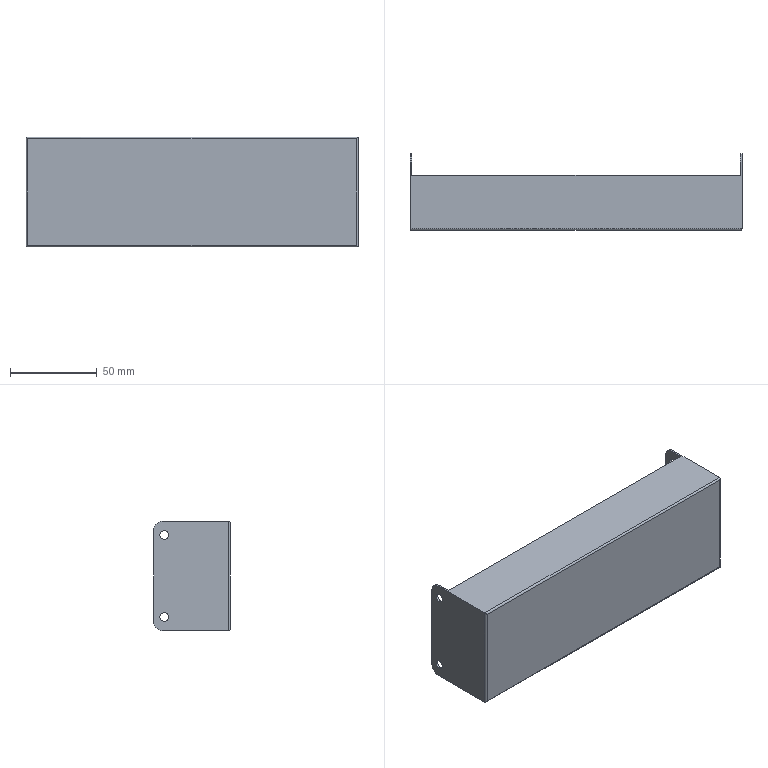Part | SolidWorks | features BaseBody 1 | 1 solid | 30 faces | box 191 x 44 x 63 mm | volume 28771 mm3 | cylinder 16 | plane 14 | commonest cylinder face diameters 5 x8 2 x4 10 x4
STEP:
#1=CARTESIAN_POINT('',(-46.937,38.,19.702));
#2=VERTEX_POINT('',#1);
#3=CARTESIAN_POINT('',(-46.937,38.,24.702));
#4=VERTEX_POINT('',#3);
#5=CARTESIAN_POINT('',(-46.937,38.,22.202));
#6=DIRECTION('',(-1.,0.,0.));
#7=DIRECTION('',(0.,0.,1.));
#8=AXIS2_PLACEMENT_3D('',#5,#6,#7);
#9=CIRCLE('',#8,2.5);
#10=EDGE_CURVE('',#2,#4,#9,.T.);
#11=ORIENTED_EDGE('',*,*,#10,.F.);
#12=CARTESIAN_POINT('',(-47.937,38.,19.702));
#13=VERTEX_POINT('',#12);
#14=CARTESIAN_POINT('',(-47.937,38.,19.702));
#15=DIRECTION('',(-1.,0.,0.));
#16=VECTOR('',#15,1000.);
#17=LINE('',#14,#16);
#18=EDGE_CURVE('',#2,#13,#17,.T.);
#19=ORIENTED_EDGE('',*,*,#18,.T.);
#20=CARTESIAN_POINT('',(-47.937,38.,24.702));
#21=VERTEX_POINT('',#20);
#22=CARTESIAN_POINT('',(-47.937,38.,22.202));
#23=DIRECTION('',(-1.,0.,0.));
#24=DIRECTION('',(0.,0.,1.));
#25=AXIS2_PLACEMENT_3D('',#22,#23,#24);
#26=CIRCLE('',#25,2.5);
#27=EDGE_CURVE('',#13,#21,#26,.T.);
#28=ORIENTED_EDGE('',*,*,#27,.T.);
#29=CARTESIAN_POINT('',(-47.937,38.,24.702));
#30=DIRECTION('',(-1.,0.,0.));
#31=VECTOR('',#30,1000.);
#32=LINE('',#29,#31);
#33=EDGE_CURVE('',#4,#21,#32,.T.);
#34=ORIENTED_EDGE('',*,*,#33,.F.);
#35=EDGE_LOOP('',(#11,#19,#28,#34));
#36=FACE_OUTER_BOUND('',#35,.T.);
#37=CARTESIAN_POINT('',(-47.937,38.,22.202));
#38=DIRECTION('',(-1.,0.,0.));
#39=DIRECTION('',(0.,0.,1.));
#40=AXIS2_PLACEMENT_3D('',#37,#38,#39);
#41=CYLINDRICAL_SURFACE('',#40,2.5);
#42=ADVANCED_FACE('',(#36),#41,.F.);
#43=CARTESIAN_POINT('',(-46.937,38.,-27.298));
#44=VERTEX_POINT('',#43);
#45=CARTESIAN_POINT('',(-46.937,38.,-22.298));
#46=VERTEX_POINT('',#45);
#47=CARTESIAN_POINT('',(-46.937,38.,-24.798));
#48=DIRECTION('',(-1.,0.,0.));
#49=DIRECTION('',(0.,0.,1.));
#50=AXIS2_PLACEMENT_3D('',#47,#48,#49);
#51=CIRCLE('',#50,2.5);
#52=EDGE_CURVE('',#44,#46,#51,.T.);
#53=ORIENTED_EDGE('',*,*,#52,.F.);
#54=CARTESIAN_POINT('',(-47.937,38.,-27.298));
#55=VERTEX_POINT('',#54);
#56=CARTESIAN_POINT('',(-47.937,38.,-27.298));
#57=DIRECTION('',(-1.,0.,0.));
#58=VECTOR('',#57,1000.);
#59=LINE('',#56,#58);
#60=EDGE_CURVE('',#44,#55,#59,.T.);
#61=ORIENTED_EDGE('',*,*,#60,.T.);
#62=CARTESIAN_POINT('',(-47.937,38.,-22.298));
#63=VERTEX_POINT('',#62);
#64=CARTESIAN_POINT('',(-47.937,38.,-24.798));
#65=DIRECTION('',(-1.,0.,0.));
#66=DIRECTION('',(0.,0.,1.));
#67=AXIS2_PLACEMENT_3D('',#64,#65,#66);
#68=CIRCLE('',#67,2.5);
#69=EDGE_CURVE('',#55,#63,#68,.T.);
#70=ORIENTED_EDGE('',*,*,#69,.T.);
#71=CARTESIAN_POINT('',(-47.937,38.,-22.298));
#72=DIRECTION('',(-1.,0.,0.));
#73=VECTOR('',#72,1000.);
#74=LINE('',#71,#73);
#75=EDGE_CURVE('',#46,#63,#74,.T.);
#76=ORIENTED_EDGE('',*,*,#75,.F.);
#77=EDGE_LOOP('',(#53,#61,#70,#76));
#78=FACE_OUTER_BOUND('',#77,.T.);
#79=CARTESIAN_POINT('',(-47.937,38.,-24.798));
#80=DIRECTION('',(-1.,0.,0.));
#81=DIRECTION('',(0.,0.,1.));
#82=AXIS2_PLACEMENT_3D('',#79,#80,#81);
#83=CYLINDRICAL_SURFACE('',#82,2.5);
#84=ADVANCED_FACE('',(#78),#83,.F.);
#85=CARTESIAN_POINT('',(143.063,38.,24.702));
#86=VERTEX_POINT('',#85);
#87=CARTESIAN_POINT('',(143.063,38.,19.702));
#88=VERTEX_POINT('',#87);
#89=CARTESIAN_POINT('',(143.063,38.,22.202));
#90=DIRECTION('',(1.,0.,0.));
#91=DIRECTION('',(0.,0.,1.));
#92=AXIS2_PLACEMENT_3D('',#89,#90,#91);
#93=CIRCLE('',#92,2.5);
#94=EDGE_CURVE('',#86,#88,#93,.T.);
#95=ORIENTED_EDGE('',*,*,#94,.T.);
#96=CARTESIAN_POINT('',(142.063,38.,19.702));
#97=VERTEX_POINT('',#96);
#98=CARTESIAN_POINT('',(-47.937,38.,19.702));
#99=DIRECTION('',(-1.,0.,0.));
#100=VECTOR('',#99,1000.);
#101=LINE('',#98,#100);
#102=EDGE_CURVE('',#88,#97,#101,.T.);
#103=ORIENTED_EDGE('',*,*,#102,.T.);
#104=CARTESIAN_POINT('',(142.063,38.,24.702));
#105=VERTEX_POINT('',#104);
#106=CARTESIAN_POINT('',(142.063,38.,22.202));
#107=DIRECTION('',(1.,0.,0.));
#108=DIRECTION('',(0.,0.,1.));
#109=AXIS2_PLACEMENT_3D('',#106,#107,#108);
#110=CIRCLE('',#109,2.5);
#111=EDGE_CURVE('',#105,#97,#110,.T.);
#112=ORIENTED_EDGE('',*,*,#111,.F.);
#113=CARTESIAN_POINT('',(-47.937,38.,24.702));
#114=DIRECTION('',(-1.,0.,0.));
#115=VECTOR('',#114,1000.);
#116=LINE('',#113,#115);
#117=EDGE_CURVE('',#86,#105,#116,.T.);
#118=ORIENTED_EDGE('',*,*,#117,.F.);
#119=EDGE_LOOP('',(#95,#103,#112,#118));
#120=FACE_OUTER_BOUND('',#119,.T.);
#121=CARTESIAN_POINT('',(-47.937,38.,22.202));
#122=DIRECTION('',(-1.,0.,0.));
#123=DIRECTION('',(0.,0.,1.));
#124=AXIS2_PLACEMENT_3D('',#121,#122,#123);
#125=CYLINDRICAL_SURFACE('',#124,2.5);
#126=ADVANCED_FACE('',(#120),#125,.F.);
#127=CARTESIAN_POINT('',(143.063,38.,-22.298));
#128=VERTEX_POINT('',#127);
#129=CARTESIAN_POINT('',(143.063,38.,-27.298));
#130=VERTEX_POINT('',#129);
#131=CARTESIAN_POINT('',(143.063,38.,-24.798));
#132=DIRECTION('',(1.,0.,0.));
#133=DIRECTION('',(0.,0.,1.));
#134=AXIS2_PLACEMENT_3D('',#131,#132,#133);
#135=CIRCLE('',#134,2.5);
#136=EDGE_CURVE('',#128,#130,#135,.T.);
#137=ORIENTED_EDGE('',*,*,#136,.T.);
#138=CARTESIAN_POINT('',(142.063,38.,-27.298));
#139=VERTEX_POINT('',#138);
#140=CARTESIAN_POINT('',(-47.937,38.,-27.298));
#141=DIRECTION('',(-1.,0.,0.));
#142=VECTOR('',#141,1000.);
#143=LINE('',#140,#142);
#144=EDGE_CURVE('',#130,#139,#143,.T.);
#145=ORIENTED_EDGE('',*,*,#144,.T.);
#146=CARTESIAN_POINT('',(142.063,38.,-22.298));
#147=VERTEX_POINT('',#146);
#148=CARTESIAN_POINT('',(142.063,38.,-24.798));
#149=DIRECTION('',(1.,0.,0.));
#150=DIRECTION('',(0.,0.,1.));
#151=AXIS2_PLACEMENT_3D('',#148,#149,#150);
#152=CIRCLE('',#151,2.5);
#153=EDGE_CURVE('',#147,#139,#152,.T.);
#154=ORIENTED_EDGE('',*,*,#153,.F.);
#155=CARTESIAN_POINT('',(-47.937,38.,-22.298));
#156=DIRECTION('',(-1.,0.,0.));
#157=VECTOR('',#156,1000.);
#158=LINE('',#155,#157);
#159=EDGE_CURVE('',#128,#147,#158,.T.);
#160=ORIENTED_EDGE('',*,*,#159,.F.);
#161=EDGE_LOOP('',(#137,#145,#154,#160));
#162=FACE_OUTER_BOUND('',#161,.T.);
#163=CARTESIAN_POINT('',(-47.937,38.,-24.798));
#164=DIRECTION('',(-1.,0.,0.));
#165=DIRECTION('',(0.,0.,1.));
#166=AXIS2_PLACEMENT_3D('',#163,#164,#165);
#167=CYLINDRICAL_SURFACE('',#166,2.5);
#168=ADVANCED_FACE('',(#162),#167,.F.);
#169=CARTESIAN_POINT('',(-46.937,0.,-31.798));
#170=VERTEX_POINT('',#169);
#171=CARTESIAN_POINT('',(-46.937,0.,29.202));
#172=VERTEX_POINT('',#171);
#173=CARTESIAN_POINT('',(-46.937,0.,0.));
#174=DIRECTION('',(0.,0.,1.));
#175=VECTOR('',#174,1000.);
#176=LINE('',#173,#175);
#177=EDGE_CURVE('',#170,#172,#176,.T.);
#178=ORIENTED_EDGE('',*,*,#177,.F.);
#179=CARTESIAN_POINT('',(142.063,0.,-31.798));
#180=VERTEX_POINT('',#179);
#181=CARTESIAN_POINT('',(0.,0.,-31.798));
#182=DIRECTION('',(-1.,0.,0.));
#183=VECTOR('',#182,1000.);
#184=LINE('',#181,#183);
#185=EDGE_CURVE('',#180,#170,#184,.T.);
#186=ORIENTED_EDGE('',*,*,#185,.F.);
#187=CARTESIAN_POINT('',(142.063,0.,29.202));
#188=VERTEX_POINT('',#187);
#189=CARTESIAN_POINT('',(142.063,0.,0.));
#190=DIRECTION('',(0.,0.,-1.));
#191=VECTOR('',#190,1000.);
#192=LINE('',#189,#191);
#193=EDGE_CURVE('',#188,#180,#192,.T.);
#194=ORIENTED_EDGE('',*,*,#193,.F.);
#195=CARTESIAN_POINT('',(0.,0.,29.202));
#196=DIRECTION('',(1.,0.,0.));
#197=VECTOR('',#196,1000.);
#198=LINE('',#195,#197);
#199=EDGE_CURVE('',#172,#188,#198,.T.);
#200=ORIENTED_EDGE('',*,*,#199,.F.);
#201=EDGE_LOOP('',(#178,#186,#194,#200));
#202=FACE_OUTER_BOUND('',#201,.T.);
#203=CARTESIAN_POINT('',(0.,0.,0.));
#204=DIRECTION('',(0.,1.,0.));
#205=DIRECTION('',(0.,0.,1.));
#206=AXIS2_PLACEMENT_3D('',#203,#204,#205);
#207=PLANE('',#206);
#208=ADVANCED_FACE('',(#202),#207,.F.);
#209=CARTESIAN_POINT('',(-47.937,1.,30.202));
#210=VERTEX_POINT('',#209);
#211=CARTESIAN_POINT('',(-47.937,1.,30.202));
#212=CARTESIAN_POINT('',(-47.937,0.4142,30.202));
#213=CARTESIAN_POINT('',(-47.523,0.,29.788));
#214=CARTESIAN_POINT('',(-46.937,0.,29.202));
#215=(BOUNDED_CURVE()B_SPLINE_CURVE(3,(#211,#212,#213,#214),.UNSPECIFIED.,.F.,.F.)B_SPLINE_CURVE_WITH_KNOTS((4,4),(3.142,4.712),.UNSPECIFIED.)CURVE()GEOMETRIC_REPRESENTATION_ITEM()RATIONAL_B_SPLINE_CURVE((1.,0.8047,0.8047,1.))REPRESENTATION_ITEM(''));
#216=EDGE_CURVE('',#210,#172,#215,.T.);
#217=ORIENTED_EDGE('',*,*,#216,.T.);
#218=ORIENTED_EDGE('',*,*,#199,.T.);
#219=CARTESIAN_POINT('',(143.063,1.,30.202));
#220=VERTEX_POINT('',#219);
#221=CARTESIAN_POINT('',(142.063,0.,29.202));
#222=CARTESIAN_POINT('',(142.649,0.,29.788));
#223=CARTESIAN_POINT('',(143.063,0.4142,30.202));
#224=CARTESIAN_POINT('',(143.063,1.,30.202));
#225=(BOUNDED_CURVE()B_SPLINE_CURVE(3,(#221,#222,#223,#224),.UNSPECIFIED.,.F.,.F.)B_SPLINE_CURVE_WITH_KNOTS((4,4),(4.712,6.283),.UNSPECIFIED.)CURVE()GEOMETRIC_REPRESENTATION_ITEM()RATIONAL_B_SPLINE_CURVE((1.,0.8047,0.8047,1.))REPRESENTATION_ITEM(''));
#226=EDGE_CURVE('',#188,#220,#225,.T.);
#227=ORIENTED_EDGE('',*,*,#226,.T.);
#228=CARTESIAN_POINT('',(-47.937,1.,30.202));
#229=DIRECTION('',(-1.,0.,0.));
#230=VECTOR('',#229,1000.);
#231=LINE('',#228,#230);
#232=EDGE_CURVE('',#220,#210,#231,.T.);
#233=ORIENTED_EDGE('',*,*,#232,.T.);
#234=EDGE_LOOP('',(#217,#218,#227,#233));
#235=FACE_OUTER_BOUND('',#234,.T.);
#236=CARTESIAN_POINT('',(-47.937,1.,29.202));
#237=DIRECTION('',(1.,0.,0.));
#238=DIRECTION('',(0.,0.,-1.));
#239=AXIS2_PLACEMENT_3D('',#236,#237,#238);
#240=CYLINDRICAL_SURFACE('',#239,1.);
#241=ADVANCED_FACE('',(#235),#240,.T.);
#242=ORIENTED_EDGE('',*,*,#216,.F.);
#243=CARTESIAN_POINT('',(-47.937,1.,-32.798));
#244=VERTEX_POINT('',#243);
#245=CARTESIAN_POINT('',(-47.937,1.,-32.798));
#246=DIRECTION('',(0.,0.,-1.));
#247=VECTOR('',#246,1000.);
#248=LINE('',#245,#247);
#249=EDGE_CURVE('',#210,#244,#248,.T.);
#250=ORIENTED_EDGE('',*,*,#249,.T.);
#251=CARTESIAN_POINT('',(-47.937,1.,-32.798));
#252=CARTESIAN_POINT('',(-47.937,0.4142,-32.798));
#253=CARTESIAN_POINT('',(-47.523,0.,-32.383));
#254=CARTESIAN_POINT('',(-46.937,0.,-31.798));
#255=(BOUNDED_CURVE()B_SPLINE_CURVE(3,(#251,#252,#253,#254),.UNSPECIFIED.,.F.,.F.)B_SPLINE_CURVE_WITH_KNOTS((4,4),(3.142,4.712),.UNSPECIFIED.)CURVE()GEOMETRIC_REPRESENTATION_ITEM()RATIONAL_B_SPLINE_CURVE((1.,0.8047,0.8047,1.))REPRESENTATION_ITEM(''));
#256=EDGE_CURVE('',#244,#170,#255,.T.);
#257=ORIENTED_EDGE('',*,*,#256,.T.);
#258=ORIENTED_EDGE('',*,*,#177,.T.);
#259=EDGE_LOOP('',(#242,#250,#257,#258));
#260=FACE_OUTER_BOUND('',#259,.T.);
#261=CARTESIAN_POINT('',(-46.937,1.,-32.798));
#262=DIRECTION('',(0.,0.,1.));
#263=DIRECTION('',(1.,0.,0.));
#264=AXIS2_PLACEMENT_3D('',#261,#262,#263);
#265=CYLINDRICAL_SURFACE('',#264,1.);
#266=ADVANCED_FACE('',(#260),#265,.T.);
#267=ORIENTED_EDGE('',*,*,#256,.F.);
#268=CARTESIAN_POINT('',(143.063,1.,-32.798));
#269=VERTEX_POINT('',#268);
#270=CARTESIAN_POINT('',(-47.937,1.,-32.798));
#271=DIRECTION('',(1.,0.,0.));
#272=VECTOR('',#271,1000.);
#273=LINE('',#270,#272);
#274=EDGE_CURVE('',#244,#269,#273,.T.);
#275=ORIENTED_EDGE('',*,*,#274,.T.);
#276=CARTESIAN_POINT('',(143.063,1.,-32.798));
#277=CARTESIAN_POINT('',(143.063,0.4142,-32.798));
#278=CARTESIAN_POINT('',(142.649,0.,-32.383));
#279=CARTESIAN_POINT('',(142.063,0.,-31.798));
#280=(BOUNDED_CURVE()B_SPLINE_CURVE(3,(#276,#277,#278,#279),.UNSPECIFIED.,.F.,.F.)B_SPLINE_CURVE_WITH_KNOTS((4,4),(3.142,4.712),.UNSPECIFIED.)CURVE()GEOMETRIC_REPRESENTATION_ITEM()RATIONAL_B_SPLINE_CURVE((1.,0.8047,0.8047,1.))REPRESENTATION_ITEM(''));
#281=EDGE_CURVE('',#269,#180,#280,.T.);
#282=ORIENTED_EDGE('',*,*,#281,.T.);
#283=ORIENTED_EDGE('',*,*,#185,.T.);
#284=EDGE_LOOP('',(#267,#275,#282,#283));
#285=FACE_OUTER_BOUND('',#284,.T.);
#286=CARTESIAN_POINT('',(-47.937,1.,-31.798));
#287=DIRECTION('',(-1.,0.,0.));
#288=DIRECTION('',(0.,0.,1.));
#289=AXIS2_PLACEMENT_3D('',#286,#287,#288);
#290=CYLINDRICAL_SURFACE('',#289,1.);
#291=ADVANCED_FACE('',(#285),#290,.T.);
#292=ORIENTED_EDGE('',*,*,#281,.F.);
#293=CARTESIAN_POINT('',(143.063,1.,-32.798));
#294=DIRECTION('',(0.,0.,1.));
#295=VECTOR('',#294,1000.);
#296=LINE('',#293,#295);
#297=EDGE_CURVE('',#269,#220,#296,.T.);
#298=ORIENTED_EDGE('',*,*,#297,.T.);
#299=ORIENTED_EDGE('',*,*,#226,.F.);
#300=ORIENTED_EDGE('',*,*,#193,.T.);
#301=EDGE_LOOP('',(#292,#298,#299,#300));
#302=FACE_OUTER_BOUND('',#301,.T.);
#303=CARTESIAN_POINT('',(142.063,1.,-32.798));
#304=DIRECTION('',(0.,0.,-1.));
#305=DIRECTION('',(-1.,0.,0.));
#306=AXIS2_PLACEMENT_3D('',#303,#304,#305);
#307=CYLINDRICAL_SURFACE('',#306,1.);
#308=ADVANCED_FACE('',(#302),#307,.T.);
#309=CARTESIAN_POINT('',(-47.937,39.,30.202));
#310=VERTEX_POINT('',#309);
#311=CARTESIAN_POINT('',(-46.937,39.,30.202));
#312=VERTEX_POINT('',#311);
#313=CARTESIAN_POINT('',(-47.937,39.,30.202));
#314=DIRECTION('',(1.,0.,0.));
#315=VECTOR('',#314,1000.);
#316=LINE('',#313,#315);
#317=EDGE_CURVE('',#310,#312,#316,.T.);
#318=ORIENTED_EDGE('',*,*,#317,.F.);
#319=CARTESIAN_POINT('',(-47.937,44.,30.202));
#320=DIRECTION('',(0.,1.,0.));
#321=VECTOR('',#320,1000.);
#322=LINE('',#319,#321);
#323=EDGE_CURVE('',#210,#310,#322,.T.);
#324=ORIENTED_EDGE('',*,*,#323,.F.);
#325=ORIENTED_EDGE('',*,*,#232,.F.);
#326=CARTESIAN_POINT('',(143.063,39.,30.202));
#327=VERTEX_POINT('',#326);
#328=CARTESIAN_POINT('',(143.063,44.,30.202));
#329=DIRECTION('',(0.,-1.,0.));
#330=VECTOR('',#329,1000.);
#331=LINE('',#328,#330);
#332=EDGE_CURVE('',#327,#220,#331,.T.);
#333=ORIENTED_EDGE('',*,*,#332,.F.);
#334=CARTESIAN_POINT('',(142.063,39.,30.202));
#335=VERTEX_POINT('',#334);
#336=CARTESIAN_POINT('',(-47.937,39.,30.202));
#337=DIRECTION('',(1.,0.,0.));
#338=VECTOR('',#337,1000.);
#339=LINE('',#336,#338);
#340=EDGE_CURVE('',#335,#327,#339,.T.);
#341=ORIENTED_EDGE('',*,*,#340,.F.);
#342=CARTESIAN_POINT('',(142.063,31.5,30.202));
#343=VERTEX_POINT('',#342);
#344=CARTESIAN_POINT('',(142.063,44.,30.202));
#345=DIRECTION('',(0.,1.,0.));
#346=VECTOR('',#345,1000.);
#347=LINE('',#344,#346);
#348=EDGE_CURVE('',#343,#335,#347,.T.);
#349=ORIENTED_EDGE('',*,*,#348,.F.);
#350=CARTESIAN_POINT('',(-46.937,31.5,30.202));
#351=VERTEX_POINT('',#350);
#352=CARTESIAN_POINT('',(-47.937,31.5,30.202));
#353=DIRECTION('',(1.,0.,0.));
#354=VECTOR('',#353,1000.);
#355=LINE('',#352,#354);
#356=EDGE_CURVE('',#351,#343,#355,.T.);
#357=ORIENTED_EDGE('',*,*,#356,.F.);
#358=CARTESIAN_POINT('',(-46.937,44.,30.202));
#359=DIRECTION('',(0.,-1.,0.));
#360=VECTOR('',#359,1000.);
#361=LINE('',#358,#360);
#362=EDGE_CURVE('',#312,#351,#361,.T.);
#363=ORIENTED_EDGE('',*,*,#362,.F.);
#364=EDGE_LOOP('',(#318,#324,#325,#333,#341,#349,#357,#363));
#365=FACE_OUTER_BOUND('',#364,.T.);
#366=CARTESIAN_POINT('',(-47.937,44.,30.202));
#367=DIRECTION('',(0.,0.,-1.));
#368=DIRECTION('',(-1.,0.,0.));
#369=AXIS2_PLACEMENT_3D('',#366,#367,#368);
#370=PLANE('',#369);
#371=ADVANCED_FACE('',(#365),#370,.F.);
#372=CARTESIAN_POINT('',(-47.937,39.,-32.798));
#373=VERTEX_POINT('',#372);
#374=CARTESIAN_POINT('',(-47.937,44.,-27.798));
#375=VERTEX_POINT('',#374);
#376=CARTESIAN_POINT('',(-47.937,39.,-27.798));
#377=DIRECTION('',(1.,0.,0.));
#378=DIRECTION('',(0.,0.,-1.));
#379=AXIS2_PLACEMENT_3D('',#376,#377,#378);
#380=CIRCLE('',#379,5.);
#381=EDGE_CURVE('',#373,#375,#380,.T.);
#382=ORIENTED_EDGE('',*,*,#381,.F.);
#383=CARTESIAN_POINT('',(-47.937,44.,-32.798));
#384=DIRECTION('',(0.,1.,0.));
#385=VECTOR('',#384,1000.);
#386=LINE('',#383,#385);
#387=EDGE_CURVE('',#244,#373,#386,.T.);
#388=ORIENTED_EDGE('',*,*,#387,.F.);
#389=ORIENTED_EDGE('',*,*,#249,.F.);
#390=ORIENTED_EDGE('',*,*,#323,.T.);
#391=CARTESIAN_POINT('',(-47.937,44.,25.202));
#392=VERTEX_POINT('',#391);
#393=CARTESIAN_POINT('',(-47.937,39.,25.202));
#394=DIRECTION('',(1.,0.,0.));
#395=DIRECTION('',(0.,0.,1.));
#396=AXIS2_PLACEMENT_3D('',#393,#394,#395);
#397=CIRCLE('',#396,5.);
#398=EDGE_CURVE('',#392,#310,#397,.T.);
#399=ORIENTED_EDGE('',*,*,#398,.F.);
#400=CARTESIAN_POINT('',(-47.937,44.,-32.798));
#401=DIRECTION('',(0.,0.,1.));
#402=VECTOR('',#401,1000.);
#403=LINE('',#400,#402);
#404=EDGE_CURVE('',#375,#392,#403,.T.);
#405=ORIENTED_EDGE('',*,*,#404,.F.);
#406=EDGE_LOOP('',(#382,#388,#389,#390,#399,#405));
#407=FACE_OUTER_BOUND('',#406,.T.);
#408=CARTESIAN_POINT('',(-47.937,38.,22.202));
#409=DIRECTION('',(-1.,0.,0.));
#410=DIRECTION('',(0.,0.,1.));
#411=AXIS2_PLACEMENT_3D('',#408,#409,#410);
#412=CIRCLE('',#411,2.5);
#413=EDGE_CURVE('',#21,#13,#412,.T.);
#414=ORIENTED_EDGE('',*,*,#413,.F.);
#415=ORIENTED_EDGE('',*,*,#27,.F.);
#416=EDGE_LOOP('',(#414,#415));
#417=FACE_BOUND('',#416,.T.);
#418=CARTESIAN_POINT('',(-47.937,38.,-24.798));
#419=DIRECTION('',(-1.,0.,0.));
#420=DIRECTION('',(0.,0.,1.));
#421=AXIS2_PLACEMENT_3D('',#418,#419,#420);
#422=CIRCLE('',#421,2.5);
#423=EDGE_CURVE('',#63,#55,#422,.T.);
#424=ORIENTED_EDGE('',*,*,#423,.F.);
#425=ORIENTED_EDGE('',*,*,#69,.F.);
#426=EDGE_LOOP('',(#424,#425));
#427=FACE_BOUND('',#426,.T.);
#428=CARTESIAN_POINT('',(-47.937,44.,-32.798));
#429=DIRECTION('',(1.,0.,0.));
#430=DIRECTION('',(0.,0.,-1.));
#431=AXIS2_PLACEMENT_3D('',#428,#429,#430);
#432=PLANE('',#431);
#433=ADVANCED_FACE('',(#407,#417,#427),#432,.F.);
#434=CARTESIAN_POINT('',(-46.937,39.,-32.798));
#435=VERTEX_POINT('',#434);
#436=CARTESIAN_POINT('',(-47.937,39.,-32.798));
#437=DIRECTION('',(-1.,0.,0.));
#438=VECTOR('',#437,1000.);
#439=LINE('',#436,#438);
#440=EDGE_CURVE('',#435,#373,#439,.T.);
#441=ORIENTED_EDGE('',*,*,#440,.F.);
#442=CARTESIAN_POINT('',(-46.937,31.5,-32.798));
#443=VERTEX_POINT('',#442);
#444=CARTESIAN_POINT('',(-46.937,44.,-32.798));
#445=DIRECTION('',(0.,1.,0.));
#446=VECTOR('',#445,1000.);
#447=LINE('',#444,#446);
#448=EDGE_CURVE('',#443,#435,#447,.T.);
#449=ORIENTED_EDGE('',*,*,#448,.F.);
#450=CARTESIAN_POINT('',(142.063,31.5,-32.798));
#451=VERTEX_POINT('',#450);
#452=CARTESIAN_POINT('',(-47.937,31.5,-32.798));
#453=DIRECTION('',(-1.,0.,0.));
#454=VECTOR('',#453,1000.);
#455=LINE('',#452,#454);
#456=EDGE_CURVE('',#451,#443,#455,.T.);
#457=ORIENTED_EDGE('',*,*,#456,.F.);
#458=CARTESIAN_POINT('',(142.063,39.,-32.798));
#459=VERTEX_POINT('',#458);
#460=CARTESIAN_POINT('',(142.063,44.,-32.798));
#461=DIRECTION('',(0.,-1.,0.));
#462=VECTOR('',#461,1000.);
#463=LINE('',#460,#462);
#464=EDGE_CURVE('',#459,#451,#463,.T.);
#465=ORIENTED_EDGE('',*,*,#464,.F.);
#466=CARTESIAN_POINT('',(143.063,39.,-32.798));
#467=VERTEX_POINT('',#466);
#468=CARTESIAN_POINT('',(-47.937,39.,-32.798));
#469=DIRECTION('',(-1.,0.,0.));
#470=VECTOR('',#469,1000.);
#471=LINE('',#468,#470);
#472=EDGE_CURVE('',#467,#459,#471,.T.);
#473=ORIENTED_EDGE('',*,*,#472,.F.);
#474=CARTESIAN_POINT('',(143.063,44.,-32.798));
#475=DIRECTION('',(0.,1.,0.));
#476=VECTOR('',#475,1000.);
#477=LINE('',#474,#476);
#478=EDGE_CURVE('',#269,#467,#477,.T.);
#479=ORIENTED_EDGE('',*,*,#478,.F.);
#480=ORIENTED_EDGE('',*,*,#274,.F.);
#481=ORIENTED_EDGE('',*,*,#387,.T.);
#482=EDGE_LOOP('',(#441,#449,#457,#465,#473,#479,#480,#481));
#483=FACE_OUTER_BOUND('',#482,.T.);
#484=CARTESIAN_POINT('',(-47.937,44.,-32.798));
#485=DIRECTION('',(0.,0.,1.));
#486=DIRECTION('',(1.,0.,0.));
#487=AXIS2_PLACEMENT_3D('',#484,#485,#486);
#488=PLANE('',#487);
#489=ADVANCED_FACE('',(#483),#488,.F.);
#490=CARTESIAN_POINT('',(143.063,44.,-27.798));
#491=VERTEX_POINT('',#490);
#492=CARTESIAN_POINT('',(143.063,39.,-27.798));
#493=DIRECTION('',(-1.,0.,0.));
#494=DIRECTION('',(0.,0.,-1.));
#495=AXIS2_PLACEMENT_3D('',#492,#493,#494);
#496=CIRCLE('',#495,5.);
#497=EDGE_CURVE('',#491,#467,#496,.T.);
#498=ORIENTED_EDGE('',*,*,#497,.F.);
#499=CARTESIAN_POINT('',(143.063,44.,25.202));
#500=VERTEX_POINT('',#499);
#501=CARTESIAN_POINT('',(143.063,44.,-32.798));
#502=DIRECTION('',(0.,0.,-1.));
#503=VECTOR('',#502,1000.);
#504=LINE('',#501,#503);
#505=EDGE_CURVE('',#500,#491,#504,.T.);
#506=ORIENTED_EDGE('',*,*,#505,.F.);
#507=CARTESIAN_POINT('',(143.063,39.,25.202));
#508=DIRECTION('',(-1.,0.,0.));
#509=DIRECTION('',(0.,0.,1.));
#510=AXIS2_PLACEMENT_3D('',#507,#508,#509);
#511=CIRCLE('',#510,5.);
#512=EDGE_CURVE('',#327,#500,#511,.T.);
#513=ORIENTED_EDGE('',*,*,#512,.F.);
#514=ORIENTED_EDGE('',*,*,#332,.T.);
#515=ORIENTED_EDGE('',*,*,#297,.F.);
#516=ORIENTED_EDGE('',*,*,#478,.T.);
#517=EDGE_LOOP('',(#498,#506,#513,#514,#515,#516));
#518=FACE_OUTER_BOUND('',#517,.T.);
#519=ORIENTED_EDGE('',*,*,#94,.F.);
#520=CARTESIAN_POINT('',(143.063,38.,22.202));
#521=DIRECTION('',(1.,0.,0.));
#522=DIRECTION('',(0.,0.,1.));
#523=AXIS2_PLACEMENT_3D('',#520,#521,#522);
#524=CIRCLE('',#523,2.5);
#525=EDGE_CURVE('',#88,#86,#524,.T.);
#526=ORIENTED_EDGE('',*,*,#525,.F.);
#527=EDGE_LOOP('',(#519,#526));
#528=FACE_BOUND('',#527,.T.);
#529=ORIENTED_EDGE('',*,*,#136,.F.);
#530=CARTESIAN_POINT('',(143.063,38.,-24.798));
#531=DIRECTION('',(1.,0.,0.));
#532=DIRECTION('',(0.,0.,1.));
#533=AXIS2_PLACEMENT_3D('',#530,#531,#532);
#534=CIRCLE('',#533,2.5);
#535=EDGE_CURVE('',#130,#128,#534,.T.);
#536=ORIENTED_EDGE('',*,*,#535,.F.);
#537=EDGE_LOOP('',(#529,#536));
#538=FACE_BOUND('',#537,.T.);
#539=CARTESIAN_POINT('',(143.063,44.,-32.798));
#540=DIRECTION('',(-1.,0.,0.));
#541=DIRECTION('',(0.,0.,1.));
#542=AXIS2_PLACEMENT_3D('',#539,#540,#541);
#543=PLANE('',#542);
#544=ADVANCED_FACE('',(#518,#528,#538),#543,.F.);
#545=CARTESIAN_POINT('',(-46.937,1.,-31.798));
#546=VERTEX_POINT('',#545);
#547=CARTESIAN_POINT('',(-46.937,31.5,-31.798));
#548=VERTEX_POINT('',#547);
#549=CARTESIAN_POINT('',(-46.937,44.,-31.798));
#550=DIRECTION('',(0.,1.,0.));
#551=VECTOR('',#550,1000.);
#552=LINE('',#549,#551);
#553=EDGE_CURVE('',#546,#548,#552,.T.);
#554=ORIENTED_EDGE('',*,*,#553,.T.);
#555=CARTESIAN_POINT('',(-46.937,31.5,-32.798));
#556=DIRECTION('',(0.,0.,-1.));
#557=VECTOR('',#556,1000.);
#558=LINE('',#555,#557);
#559=EDGE_CURVE('',#548,#443,#558,.T.);
#560=ORIENTED_EDGE('',*,*,#559,.T.);
#561=ORIENTED_EDGE('',*,*,#448,.T.);
#562=CARTESIAN_POINT('',(-46.937,44.,-27.798));
#563=VERTEX_POINT('',#562);
#564=CARTESIAN_POINT('',(-46.937,39.,-27.798));
#565=DIRECTION('',(1.,0.,0.));
#566=DIRECTION('',(0.,0.,-1.));
#567=AXIS2_PLACEMENT_3D('',#564,#565,#566);
#568=CIRCLE('',#567,5.);
#569=EDGE_CURVE('',#435,#563,#568,.T.);
#570=ORIENTED_EDGE('',*,*,#569,.T.);
#571=CARTESIAN_POINT('',(-46.937,44.,25.202));
#572=VERTEX_POINT('',#571);
#573=CARTESIAN_POINT('',(-46.937,44.,-32.798));
#574=DIRECTION('',(0.,0.,1.));
#575=VECTOR('',#574,1000.);
#576=LINE('',#573,#575);
#577=EDGE_CURVE('',#563,#572,#576,.T.);
#578=ORIENTED_EDGE('',*,*,#577,.T.);
#579=CARTESIAN_POINT('',(-46.937,39.,25.202));
#580=DIRECTION('',(1.,0.,0.));
#581=DIRECTION('',(0.,0.,1.));
#582=AXIS2_PLACEMENT_3D('',#579,#580,#581);
#583=CIRCLE('',#582,5.);
#584=EDGE_CURVE('',#572,#312,#583,.T.);
#585=ORIENTED_EDGE('',*,*,#584,.T.);
#586=ORIENTED_EDGE('',*,*,#362,.T.);
#587=CARTESIAN_POINT('',(-46.937,31.5,29.202));
#588=VERTEX_POINT('',#587);
#589=CARTESIAN_POINT('',(-46.937,31.5,-32.798));
#590=DIRECTION('',(0.,0.,-1.));
#591=VECTOR('',#590,1000.);
#592=LINE('',#589,#591);
#593=EDGE_CURVE('',#351,#588,#592,.T.);
#594=ORIENTED_EDGE('',*,*,#593,.T.);
#595=CARTESIAN_POINT('',(-46.937,1.,29.202));
#596=VERTEX_POINT('',#595);
#597=CARTESIAN_POINT('',(-46.937,44.,29.202));
#598=DIRECTION('',(0.,-1.,0.));
#599=VECTOR('',#598,1000.);
#600=LINE('',#597,#599);
#601=EDGE_CURVE('',#588,#596,#600,.T.);
#602=ORIENTED_EDGE('',*,*,#601,.T.);
#603=CARTESIAN_POINT('',(-46.937,1.,-32.798));
#604=DIRECTION('',(0.,0.,-1.));
#605=VECTOR('',#604,1000.);
#606=LINE('',#603,#605);
#607=EDGE_CURVE('',#596,#546,#606,.T.);
#608=ORIENTED_EDGE('',*,*,#607,.T.);
#609=EDGE_LOOP('',(#554,#560,#561,#570,#578,#585,#586,#594,#602,#608));
#610=FACE_OUTER_BOUND('',#609,.T.);
#611=CARTESIAN_POINT('',(-46.937,38.,22.202));
#612=DIRECTION('',(-1.,0.,0.));
#613=DIRECTION('',(0.,0.,1.));
#614=AXIS2_PLACEMENT_3D('',#611,#612,#613);
#615=CIRCLE('',#614,2.5);
#616=EDGE_CURVE('',#4,#2,#615,.T.);
#617=ORIENTED_EDGE('',*,*,#616,.T.);
#618=ORIENTED_EDGE('',*,*,#10,.T.);
#619=EDGE_LOOP('',(#617,#618));
#620=FACE_BOUND('',#619,.T.);
#621=CARTESIAN_POINT('',(-46.937,38.,-24.798));
#622=DIRECTION('',(-1.,0.,0.));
#623=DIRECTION('',(0.,0.,1.));
#624=AXIS2_PLACEMENT_3D('',#621,#622,#623);
#625=CIRCLE('',#624,2.5);
#626=EDGE_CURVE('',#46,#44,#625,.T.);
#627=ORIENTED_EDGE('',*,*,#626,.T.);
#628=ORIENTED_EDGE('',*,*,#52,.T.);
#629=EDGE_LOOP('',(#627,#628));
#630=FACE_BOUND('',#629,.T.);
#631=CARTESIAN_POINT('',(-46.937,44.,-32.798));
#632=DIRECTION('',(1.,0.,0.));
#633=DIRECTION('',(0.,0.,-1.));
#634=AXIS2_PLACEMENT_3D('',#631,#632,#633);
#635=PLANE('',#634);
#636=ADVANCED_FACE('',(#610,#620,#630),#635,.T.);
#637=ORIENTED_EDGE('',*,*,#584,.F.);
#638=CARTESIAN_POINT('',(0.,44.,25.202));
#639=DIRECTION('',(-1.,0.,0.));
#640=VECTOR('',#639,1000.);
#641=LINE('',#638,#640);
#642=EDGE_CURVE('',#572,#392,#641,.T.);
#643=ORIENTED_EDGE('',*,*,#642,.T.);
#644=ORIENTED_EDGE('',*,*,#398,.T.);
#645=ORIENTED_EDGE('',*,*,#317,.T.);
#646=EDGE_LOOP('',(#637,#643,#644,#645));
#647=FACE_OUTER_BOUND('',#646,.T.);
#648=CARTESIAN_POINT('',(0.,39.,25.202));
#649=DIRECTION('',(-1.,0.,0.));
#650=DIRECTION('',(0.,0.,1.));
#651=AXIS2_PLACEMENT_3D('',#648,#649,#650);
#652=CYLINDRICAL_SURFACE('',#651,5.);
#653=ADVANCED_FACE('',(#647),#652,.T.);
#654=ORIENTED_EDGE('',*,*,#512,.T.);
#655=CARTESIAN_POINT('',(142.063,44.,25.202));
#656=VERTEX_POINT('',#655);
#657=CARTESIAN_POINT('',(0.,44.,25.202));
#658=DIRECTION('',(-1.,0.,0.));
#659=VECTOR('',#658,1000.);
#660=LINE('',#657,#659);
#661=EDGE_CURVE('',#500,#656,#660,.T.);
#662=ORIENTED_EDGE('',*,*,#661,.T.);
#663=CARTESIAN_POINT('',(142.063,39.,25.202));
#664=DIRECTION('',(1.,0.,0.));
#665=DIRECTION('',(0.,0.,1.));
#666=AXIS2_PLACEMENT_3D('',#663,#664,#665);
#667=CIRCLE('',#666,5.);
#668=EDGE_CURVE('',#656,#335,#667,.T.);
#669=ORIENTED_EDGE('',*,*,#668,.T.);
#670=ORIENTED_EDGE('',*,*,#340,.T.);
#671=EDGE_LOOP('',(#654,#662,#669,#670));
#672=FACE_OUTER_BOUND('',#671,.T.);
#673=CARTESIAN_POINT('',(0.,39.,25.202));
#674=DIRECTION('',(-1.,0.,0.));
#675=DIRECTION('',(0.,0.,1.));
#676=AXIS2_PLACEMENT_3D('',#673,#674,#675);
#677=CYLINDRICAL_SURFACE('',#676,5.);
#678=ADVANCED_FACE('',(#672),#677,.T.);
#679=ORIENTED_EDGE('',*,*,#348,.T.);
#680=ORIENTED_EDGE('',*,*,#668,.F.);
#681=CARTESIAN_POINT('',(142.063,44.,-27.798));
#682=VERTEX_POINT('',#681);
#683=CARTESIAN_POINT('',(142.063,44.,-32.798));
#684=DIRECTION('',(0.,0.,-1.));
#685=VECTOR('',#684,1000.);
#686=LINE('',#683,#685);
#687=EDGE_CURVE('',#656,#682,#686,.T.);
#688=ORIENTED_EDGE('',*,*,#687,.T.);
#689=CARTESIAN_POINT('',(142.063,39.,-27.798));
#690=DIRECTION('',(-1.,0.,0.));
#691=DIRECTION('',(0.,0.,-1.));
#692=AXIS2_PLACEMENT_3D('',#689,#690,#691);
#693=CIRCLE('',#692,5.);
#694=EDGE_CURVE('',#682,#459,#693,.T.);
#695=ORIENTED_EDGE('',*,*,#694,.T.);
#696=ORIENTED_EDGE('',*,*,#464,.T.);
#697=CARTESIAN_POINT('',(142.063,31.5,-31.798));
#698=VERTEX_POINT('',#697);
#699=CARTESIAN_POINT('',(142.063,31.5,-32.798));
#700=DIRECTION('',(0.,0.,1.));
#701=VECTOR('',#700,1000.);
#702=LINE('',#699,#701);
#703=EDGE_CURVE('',#451,#698,#702,.T.);
#704=ORIENTED_EDGE('',*,*,#703,.T.);
#705=CARTESIAN_POINT('',(142.063,1.,-31.798));
#706=VERTEX_POINT('',#705);
#707=CARTESIAN_POINT('',(142.063,44.,-31.798));
#708=DIRECTION('',(0.,-1.,0.));
#709=VECTOR('',#708,1000.);
#710=LINE('',#707,#709);
#711=EDGE_CURVE('',#698,#706,#710,.T.);
#712=ORIENTED_EDGE('',*,*,#711,.T.);
#713=CARTESIAN_POINT('',(142.063,1.,29.202));
#714=VERTEX_POINT('',#713);
#715=CARTESIAN_POINT('',(142.063,1.,-32.798));
#716=DIRECTION('',(0.,0.,1.));
#717=VECTOR('',#716,1000.);
#718=LINE('',#715,#717);
#719=EDGE_CURVE('',#706,#714,#718,.T.);
#720=ORIENTED_EDGE('',*,*,#719,.T.);
#721=CARTESIAN_POINT('',(142.063,31.5,29.202));
#722=VERTEX_POINT('',#721);
#723=CARTESIAN_POINT('',(142.063,44.,29.202));
#724=DIRECTION('',(0.,1.,0.));
#725=VECTOR('',#724,1000.);
#726=LINE('',#723,#725);
#727=EDGE_CURVE('',#714,#722,#726,.T.);
#728=ORIENTED_EDGE('',*,*,#727,.T.);
#729=CARTESIAN_POINT('',(142.063,31.5,-32.798));
#730=DIRECTION('',(0.,0.,1.));
#731=VECTOR('',#730,1000.);
#732=LINE('',#729,#731);
#733=EDGE_CURVE('',#722,#343,#732,.T.);
#734=ORIENTED_EDGE('',*,*,#733,.T.);
#735=EDGE_LOOP('',(#679,#680,#688,#695,#696,#704,#712,#720,#728,#734));
#736=FACE_OUTER_BOUND('',#735,.T.);
#737=ORIENTED_EDGE('',*,*,#111,.T.);
#738=CARTESIAN_POINT('',(142.063,38.,22.202));
#739=DIRECTION('',(1.,0.,0.));
#740=DIRECTION('',(0.,0.,1.));
#741=AXIS2_PLACEMENT_3D('',#738,#739,#740);
#742=CIRCLE('',#741,2.5);
#743=EDGE_CURVE('',#97,#105,#742,.T.);
#744=ORIENTED_EDGE('',*,*,#743,.T.);
#745=EDGE_LOOP('',(#737,#744));
#746=FACE_BOUND('',#745,.T.);
#747=ORIENTED_EDGE('',*,*,#153,.T.);
#748=CARTESIAN_POINT('',(142.063,38.,-24.798));
#749=DIRECTION('',(1.,0.,0.));
#750=DIRECTION('',(0.,0.,1.));
#751=AXIS2_PLACEMENT_3D('',#748,#749,#750);
#752=CIRCLE('',#751,2.5);
#753=EDGE_CURVE('',#139,#147,#752,.T.);
#754=ORIENTED_EDGE('',*,*,#753,.T.);
#755=EDGE_LOOP('',(#747,#754));
#756=FACE_BOUND('',#755,.T.);
#757=CARTESIAN_POINT('',(142.063,44.,-32.798));
#758=DIRECTION('',(-1.,0.,0.));
#759=DIRECTION('',(0.,0.,1.));
#760=AXIS2_PLACEMENT_3D('',#757,#758,#759);
#761=PLANE('',#760);
#762=ADVANCED_FACE('',(#736,#746,#756),#761,.T.);
#763=CARTESIAN_POINT('',(-46.937,31.5,29.202));
#764=DIRECTION('',(1.,0.,0.));
#765=VECTOR('',#764,1000.);
#766=LINE('',#763,#765);
#767=EDGE_CURVE('',#588,#722,#766,.T.);
#768=ORIENTED_EDGE('',*,*,#767,.F.);
#769=ORIENTED_EDGE('',*,*,#593,.F.);
#770=ORIENTED_EDGE('',*,*,#356,.T.);
#771=ORIENTED_EDGE('',*,*,#733,.F.);
#772=EDGE_LOOP('',(#768,#769,#770,#771));
#773=FACE_OUTER_BOUND('',#772,.T.);
#774=CARTESIAN_POINT('',(-46.937,31.5,67.202));
#775=DIRECTION('',(0.,-1.,0.));
#776=DIRECTION('',(1.,0.,0.));
#777=AXIS2_PLACEMENT_3D('',#774,#775,#776);
#778=PLANE('',#777);
#779=ADVANCED_FACE('',(#773),#778,.F.);
#780=ORIENTED_EDGE('',*,*,#404,.T.);
#781=ORIENTED_EDGE('',*,*,#642,.F.);
#782=ORIENTED_EDGE('',*,*,#577,.F.);
#783=CARTESIAN_POINT('',(0.,44.,-27.798));
#784=DIRECTION('',(-1.,0.,0.));
#785=VECTOR('',#784,1000.);
#786=LINE('',#783,#785);
#787=EDGE_CURVE('',#563,#375,#786,.T.);
#788=ORIENTED_EDGE('',*,*,#787,.T.);
#789=EDGE_LOOP('',(#780,#781,#782,#788));
#790=FACE_OUTER_BOUND('',#789,.T.);
#791=CARTESIAN_POINT('',(0.,44.,0.));
#792=DIRECTION('',(0.,1.,0.));
#793=DIRECTION('',(0.,0.,1.));
#794=AXIS2_PLACEMENT_3D('',#791,#792,#793);
#795=PLANE('',#794);
#796=ADVANCED_FACE('',(#790),#795,.T.);
#797=ORIENTED_EDGE('',*,*,#381,.T.);
#798=ORIENTED_EDGE('',*,*,#787,.F.);
#799=ORIENTED_EDGE('',*,*,#569,.F.);
#800=ORIENTED_EDGE('',*,*,#440,.T.);
#801=EDGE_LOOP('',(#797,#798,#799,#800));
#802=FACE_OUTER_BOUND('',#801,.T.);
#803=CARTESIAN_POINT('',(0.,39.,-27.798));
#804=DIRECTION('',(1.,0.,0.));
#805=DIRECTION('',(0.,0.,-1.));
#806=AXIS2_PLACEMENT_3D('',#803,#804,#805);
#807=CYLINDRICAL_SURFACE('',#806,5.);
#808=ADVANCED_FACE('',(#802),#807,.T.);
#809=ORIENTED_EDGE('',*,*,#18,.F.);
#810=ORIENTED_EDGE('',*,*,#616,.F.);
#811=ORIENTED_EDGE('',*,*,#33,.T.);
#812=ORIENTED_EDGE('',*,*,#413,.T.);
#813=EDGE_LOOP('',(#809,#810,#811,#812));
#814=FACE_OUTER_BOUND('',#813,.T.);
#815=CARTESIAN_POINT('',(-47.937,38.,22.202));
#816=DIRECTION('',(-1.,0.,0.));
#817=DIRECTION('',(0.,0.,1.));
#818=AXIS2_PLACEMENT_3D('',#815,#816,#817);
#819=CYLINDRICAL_SURFACE('',#818,2.5);
#820=ADVANCED_FACE('',(#814),#819,.F.);
#821=ORIENTED_EDGE('',*,*,#60,.F.);
#822=ORIENTED_EDGE('',*,*,#626,.F.);
#823=ORIENTED_EDGE('',*,*,#75,.T.);
#824=ORIENTED_EDGE('',*,*,#423,.T.);
#825=EDGE_LOOP('',(#821,#822,#823,#824));
#826=FACE_OUTER_BOUND('',#825,.T.);
#827=CARTESIAN_POINT('',(-47.937,38.,-24.798));
#828=DIRECTION('',(-1.,0.,0.));
#829=DIRECTION('',(0.,0.,1.));
#830=AXIS2_PLACEMENT_3D('',#827,#828,#829);
#831=CYLINDRICAL_SURFACE('',#830,2.5);
#832=ADVANCED_FACE('',(#826),#831,.F.);
#833=ORIENTED_EDGE('',*,*,#703,.F.);
#834=ORIENTED_EDGE('',*,*,#456,.T.);
#835=ORIENTED_EDGE('',*,*,#559,.F.);
#836=CARTESIAN_POINT('',(-46.937,31.5,-31.798));
#837=DIRECTION('',(-1.,0.,0.));
#838=VECTOR('',#837,1000.);
#839=LINE('',#836,#838);
#840=EDGE_CURVE('',#698,#548,#839,.T.);
#841=ORIENTED_EDGE('',*,*,#840,.F.);
#842=EDGE_LOOP('',(#833,#834,#835,#841));
#843=FACE_OUTER_BOUND('',#842,.T.);
#844=CARTESIAN_POINT('',(-46.937,31.5,67.202));
#845=DIRECTION('',(0.,-1.,0.));
#846=DIRECTION('',(1.,0.,0.));
#847=AXIS2_PLACEMENT_3D('',#844,#845,#846);
#848=PLANE('',#847);
#849=ADVANCED_FACE('',(#843),#848,.F.);
#850=ORIENTED_EDGE('',*,*,#694,.F.);
#851=CARTESIAN_POINT('',(0.,44.,-27.798));
#852=DIRECTION('',(1.,0.,0.));
#853=VECTOR('',#852,1000.);
#854=LINE('',#851,#853);
#855=EDGE_CURVE('',#682,#491,#854,.T.);
#856=ORIENTED_EDGE('',*,*,#855,.T.);
#857=ORIENTED_EDGE('',*,*,#497,.T.);
#858=ORIENTED_EDGE('',*,*,#472,.T.);
#859=EDGE_LOOP('',(#850,#856,#857,#858));
#860=FACE_OUTER_BOUND('',#859,.T.);
#861=CARTESIAN_POINT('',(0.,39.,-27.798));
#862=DIRECTION('',(1.,0.,0.));
#863=DIRECTION('',(0.,0.,-1.));
#864=AXIS2_PLACEMENT_3D('',#861,#862,#863);
#865=CYLINDRICAL_SURFACE('',#864,5.);
#866=ADVANCED_FACE('',(#860),#865,.T.);
#867=ORIENTED_EDGE('',*,*,#687,.F.);
#868=ORIENTED_EDGE('',*,*,#661,.F.);
#869=ORIENTED_EDGE('',*,*,#505,.T.);
#870=ORIENTED_EDGE('',*,*,#855,.F.);
#871=EDGE_LOOP('',(#867,#868,#869,#870));
#872=FACE_OUTER_BOUND('',#871,.T.);
#873=CARTESIAN_POINT('',(0.,44.,0.));
#874=DIRECTION('',(0.,1.,0.));
#875=DIRECTION('',(0.,0.,1.));
#876=AXIS2_PLACEMENT_3D('',#873,#874,#875);
#877=PLANE('',#876);
#878=ADVANCED_FACE('',(#872),#877,.T.);
#879=ORIENTED_EDGE('',*,*,#102,.F.);
#880=ORIENTED_EDGE('',*,*,#525,.T.);
#881=ORIENTED_EDGE('',*,*,#117,.T.);
#882=ORIENTED_EDGE('',*,*,#743,.F.);
#883=EDGE_LOOP('',(#879,#880,#881,#882));
#884=FACE_OUTER_BOUND('',#883,.T.);
#885=CARTESIAN_POINT('',(-47.937,38.,22.202));
#886=DIRECTION('',(-1.,0.,0.));
#887=DIRECTION('',(0.,0.,1.));
#888=AXIS2_PLACEMENT_3D('',#885,#886,#887);
#889=CYLINDRICAL_SURFACE('',#888,2.5);
#890=ADVANCED_FACE('',(#884),#889,.F.);
#891=ORIENTED_EDGE('',*,*,#144,.F.);
#892=ORIENTED_EDGE('',*,*,#535,.T.);
#893=ORIENTED_EDGE('',*,*,#159,.T.);
#894=ORIENTED_EDGE('',*,*,#753,.F.);
#895=EDGE_LOOP('',(#891,#892,#893,#894));
#896=FACE_OUTER_BOUND('',#895,.T.);
#897=CARTESIAN_POINT('',(-47.937,38.,-24.798));
#898=DIRECTION('',(-1.,0.,0.));
#899=DIRECTION('',(0.,0.,1.));
#900=AXIS2_PLACEMENT_3D('',#897,#898,#899);
#901=CYLINDRICAL_SURFACE('',#900,2.5);
#902=ADVANCED_FACE('',(#896),#901,.F.);
#903=CARTESIAN_POINT('',(-47.937,1.,-31.798));
#904=DIRECTION('',(1.,0.,0.));
#905=VECTOR('',#904,1000.);
#906=LINE('',#903,#905);
#907=EDGE_CURVE('',#546,#706,#906,.T.);
#908=ORIENTED_EDGE('',*,*,#907,.T.);
#909=ORIENTED_EDGE('',*,*,#711,.F.);
#910=ORIENTED_EDGE('',*,*,#840,.T.);
#911=ORIENTED_EDGE('',*,*,#553,.F.);
#912=EDGE_LOOP('',(#908,#909,#910,#911));
#913=FACE_OUTER_BOUND('',#912,.T.);
#914=CARTESIAN_POINT('',(-47.937,44.,-31.798));
#915=DIRECTION('',(0.,0.,1.));
#916=DIRECTION('',(1.,0.,0.));
#917=AXIS2_PLACEMENT_3D('',#914,#915,#916);
#918=PLANE('',#917);
#919=ADVANCED_FACE('',(#913),#918,.T.);
#920=ORIENTED_EDGE('',*,*,#719,.F.);
#921=ORIENTED_EDGE('',*,*,#907,.F.);
#922=ORIENTED_EDGE('',*,*,#607,.F.);
#923=CARTESIAN_POINT('',(0.,1.,29.202));
#924=DIRECTION('',(1.,0.,0.));
#925=VECTOR('',#924,1000.);
#926=LINE('',#923,#925);
#927=EDGE_CURVE('',#596,#714,#926,.T.);
#928=ORIENTED_EDGE('',*,*,#927,.T.);
#929=EDGE_LOOP('',(#920,#921,#922,#928));
#930=FACE_OUTER_BOUND('',#929,.T.);
#931=CARTESIAN_POINT('',(0.,1.,0.));
#932=DIRECTION('',(0.,1.,0.));
#933=DIRECTION('',(0.,0.,1.));
#934=AXIS2_PLACEMENT_3D('',#931,#932,#933);
#935=PLANE('',#934);
#936=ADVANCED_FACE('',(#930),#935,.T.);
#937=ORIENTED_EDGE('',*,*,#927,.F.);
#938=ORIENTED_EDGE('',*,*,#601,.F.);
#939=ORIENTED_EDGE('',*,*,#767,.T.);
#940=ORIENTED_EDGE('',*,*,#727,.F.);
#941=EDGE_LOOP('',(#937,#938,#939,#940));
#942=FACE_OUTER_BOUND('',#941,.T.);
#943=CARTESIAN_POINT('',(-47.937,44.,29.202));
#944=DIRECTION('',(0.,0.,-1.));
#945=DIRECTION('',(-1.,0.,0.));
#946=AXIS2_PLACEMENT_3D('',#943,#944,#945);
#947=PLANE('',#946);
#948=ADVANCED_FACE('',(#942),#947,.T.);
#949=CLOSED_SHELL('',(#42,#84,#126,#168,#208,#241,#266,#291,#308,#371,#433,#489,#544,#636,#653,#678,#762,#779,#796,#808,#820,#832,#849,#866,#878,#890,#902,#919,#936,#948));
#950=MANIFOLD_SOLID_BREP('',#949);
#951=CARTESIAN_POINT('',(0.,0.,0.));
#952=DIRECTION('',(0.,0.,1.));
#953=DIRECTION('',(1.,0.,0.));
#954=AXIS2_PLACEMENT_3D('',#951,#952,#953);
#955=(LENGTH_UNIT()NAMED_UNIT(*)SI_UNIT(.MILLI.,.METRE.));
#956=UNCERTAINTY_MEASURE_WITH_UNIT(LENGTH_MEASURE(0.00001),#955,'','');
#957=(NAMED_UNIT(*)PLANE_ANGLE_UNIT()SI_UNIT($,.RADIAN.));
#958=(NAMED_UNIT(*)SI_UNIT($,.STERADIAN.)SOLID_ANGLE_UNIT());
#959=(GEOMETRIC_REPRESENTATION_CONTEXT(3)GLOBAL_UNCERTAINTY_ASSIGNED_CONTEXT((#956))GLOBAL_UNIT_ASSIGNED_CONTEXT((#955,#957,#958))REPRESENTATION_CONTEXT('',''));
#960=ADVANCED_BREP_SHAPE_REPRESENTATION('',(#950,#954),#959);